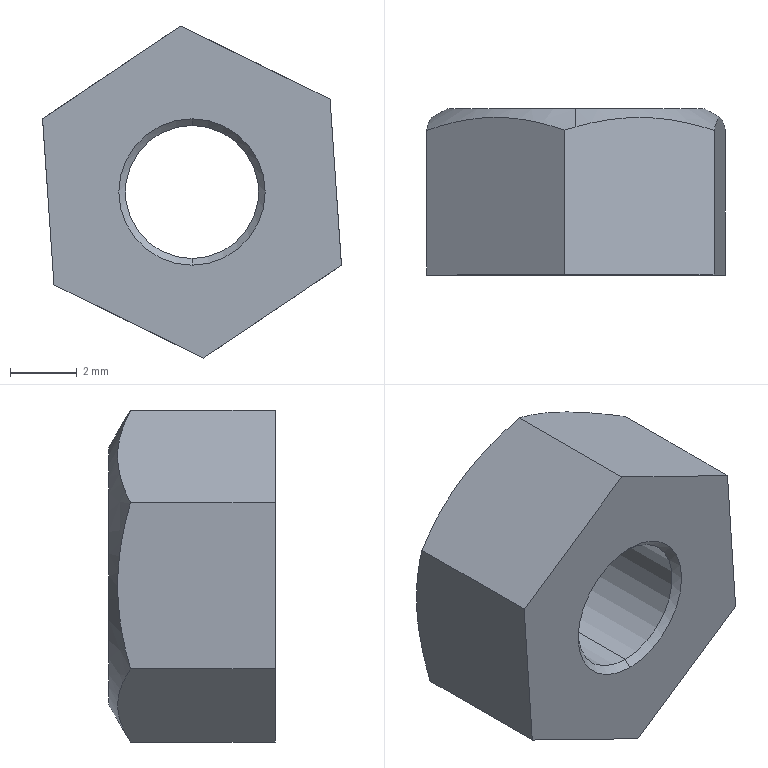Part | SolidWorks | features Chamfer 2, Extrusion 1, ICE 1 | 1 solid | 16 faces | box 8.983 x 5 x 9.976 mm | volume 257.478 mm3 | plane 8 | cone 6 | cylinder 2 | commonest cylinder face diameters 4 x2
STEP:
#1=CARTESIAN_POINT('',(0.,0.007874,0.07874));
#2=VERTEX_POINT('',#1);
#3=CARTESIAN_POINT('',(0.,0.007874,-0.07874));
#4=VERTEX_POINT('',#3);
#5=CARTESIAN_POINT('',(0.,0.007874,0.));
#6=DIRECTION('',(0.,-1.,0.));
#7=DIRECTION('',(0.,0.,1.));
#8=AXIS2_PLACEMENT_3D('',#5,#6,#7);
#9=CIRCLE('',#8,0.07874);
#10=EDGE_CURVE('',#2,#4,#9,.T.);
#11=ORIENTED_EDGE('',*,*,#10,.F.);
#12=CARTESIAN_POINT('',(0.,0.,0.08661));
#13=VERTEX_POINT('',#12);
#14=CARTESIAN_POINT('',(0.,0.,0.08661));
#15=DIRECTION('',(0.,-0.7071,0.7071));
#16=VECTOR('',#15,39.37);
#17=LINE('',#14,#16);
#18=EDGE_CURVE('',#2,#13,#17,.T.);
#19=ORIENTED_EDGE('',*,*,#18,.T.);
#20=CARTESIAN_POINT('',(0.,0.,-0.08661));
#21=VERTEX_POINT('',#20);
#22=CARTESIAN_POINT('',(0.,0.,0.));
#23=DIRECTION('',(0.,1.,0.));
#24=DIRECTION('',(0.,0.,1.));
#25=AXIS2_PLACEMENT_3D('',#22,#23,#24);
#26=CIRCLE('',#25,0.08661);
#27=EDGE_CURVE('',#21,#13,#26,.T.);
#28=ORIENTED_EDGE('',*,*,#27,.F.);
#29=CARTESIAN_POINT('',(0.,0.,-0.08661));
#30=DIRECTION('',(0.,-0.7071,-0.7071));
#31=VECTOR('',#30,39.37);
#32=LINE('',#29,#31);
#33=EDGE_CURVE('',#4,#21,#32,.T.);
#34=ORIENTED_EDGE('',*,*,#33,.F.);
#35=EDGE_LOOP('',(#11,#19,#28,#34));
#36=FACE_OUTER_BOUND('',#35,.T.);
#37=CARTESIAN_POINT('',(0.,0.,0.));
#38=DIRECTION('',(0.,-1.,0.));
#39=DIRECTION('',(0.,0.,-1.));
#40=AXIS2_PLACEMENT_3D('',#37,#38,#39);
#41=CONICAL_SURFACE('',#40,0.08661,0.7854);
#42=ADVANCED_FACE('',(#36),#41,.F.);
#43=CARTESIAN_POINT('',(0.,0.189,-0.07874));
#44=VERTEX_POINT('',#43);
#45=CARTESIAN_POINT('',(0.,0.189,0.07874));
#46=VERTEX_POINT('',#45);
#47=CARTESIAN_POINT('',(0.,0.189,0.));
#48=DIRECTION('',(0.,1.,0.));
#49=DIRECTION('',(0.,0.,1.));
#50=AXIS2_PLACEMENT_3D('',#47,#48,#49);
#51=CIRCLE('',#50,0.07874);
#52=EDGE_CURVE('',#44,#46,#51,.T.);
#53=ORIENTED_EDGE('',*,*,#52,.F.);
#54=CARTESIAN_POINT('',(0.,0.1969,-0.08661));
#55=VERTEX_POINT('',#54);
#56=CARTESIAN_POINT('',(0.,0.189,-0.07874));
#57=DIRECTION('',(0.,0.7071,-0.7071));
#58=VECTOR('',#57,39.37);
#59=LINE('',#56,#58);
#60=EDGE_CURVE('',#44,#55,#59,.T.);
#61=ORIENTED_EDGE('',*,*,#60,.T.);
#62=CARTESIAN_POINT('',(0.,0.1969,0.08661));
#63=VERTEX_POINT('',#62);
#64=CARTESIAN_POINT('',(0.,0.1969,0.));
#65=DIRECTION('',(0.,-1.,0.));
#66=DIRECTION('',(0.,0.,1.));
#67=AXIS2_PLACEMENT_3D('',#64,#65,#66);
#68=CIRCLE('',#67,0.08661);
#69=EDGE_CURVE('',#63,#55,#68,.T.);
#70=ORIENTED_EDGE('',*,*,#69,.F.);
#71=CARTESIAN_POINT('',(0.,0.189,0.07874));
#72=DIRECTION('',(0.,0.7071,0.7071));
#73=VECTOR('',#72,39.37);
#74=LINE('',#71,#73);
#75=EDGE_CURVE('',#46,#63,#74,.T.);
#76=ORIENTED_EDGE('',*,*,#75,.F.);
#77=EDGE_LOOP('',(#53,#61,#70,#76));
#78=FACE_OUTER_BOUND('',#77,.T.);
#79=CARTESIAN_POINT('',(0.,0.189,0.));
#80=DIRECTION('',(0.,1.,0.));
#81=DIRECTION('',(0.,0.,1.));
#82=AXIS2_PLACEMENT_3D('',#79,#80,#81);
#83=CONICAL_SURFACE('',#82,0.07874,0.7854);
#84=ADVANCED_FACE('',(#78),#83,.F.);
#85=CARTESIAN_POINT('',(0.,0.1969,-0.1523));
#86=VERTEX_POINT('',#85);
#87=CARTESIAN_POINT('',(0.,0.1969,0.1523));
#88=VERTEX_POINT('',#87);
#89=CARTESIAN_POINT('',(0.,0.1969,0.));
#90=DIRECTION('',(0.,1.,0.));
#91=DIRECTION('',(0.,0.,1.));
#92=AXIS2_PLACEMENT_3D('',#89,#90,#91);
#93=CIRCLE('',#92,0.1523);
#94=EDGE_CURVE('',#86,#88,#93,.T.);
#95=ORIENTED_EDGE('',*,*,#94,.F.);
#96=CARTESIAN_POINT('',(0.,0.1752,-0.1898));
#97=VERTEX_POINT('',#96);
#98=CARTESIAN_POINT('',(0.,0.1969,-0.1523));
#99=DIRECTION('',(0.,-0.5,-0.866));
#100=VECTOR('',#99,39.37);
#101=LINE('',#98,#100);
#102=EDGE_CURVE('',#86,#97,#101,.T.);
#103=ORIENTED_EDGE('',*,*,#102,.T.);
#104=CARTESIAN_POINT('',(-0.1633,0.1711,-0.1099));
#105=VERTEX_POINT('',#104);
#106=CARTESIAN_POINT('',(0.,0.1752,-0.1898));
#107=CARTESIAN_POINT('',(-0.02676,0.1828,-0.1767));
#108=CARTESIAN_POINT('',(-0.05395,0.1871,-0.1634));
#109=CARTESIAN_POINT('',(-0.1096,0.1855,-0.1362));
#110=CARTESIAN_POINT('',(-0.1367,0.1797,-0.1229));
#111=CARTESIAN_POINT('',(-0.1633,0.1711,-0.1099));
#112=B_SPLINE_CURVE_WITH_KNOTS('',3,(#106,#107,#108,#109,#110,#111),.UNSPECIFIED.,.F.,.F.,(4,2,4),(0.0003933,0.002722,0.00505),.UNSPECIFIED.);
#113=EDGE_CURVE('',#97,#105,#112,.T.);
#114=ORIENTED_EDGE('',*,*,#113,.T.);
#115=CARTESIAN_POINT('',(-0.1768,0.1711,0.08649));
#116=VERTEX_POINT('',#115);
#117=CARTESIAN_POINT('',(-0.1633,0.1711,-0.1099));
#118=CARTESIAN_POINT('',(-0.1655,0.1804,-0.07783));
#119=CARTESIAN_POINT('',(-0.1678,0.1863,-0.04529));
#120=CARTESIAN_POINT('',(-0.1712,0.1864,0.004801));
#121=CARTESIAN_POINT('',(-0.1724,0.1849,0.02148));
#122=CARTESIAN_POINT('',(-0.1746,0.1796,0.05425));
#123=CARTESIAN_POINT('',(-0.1757,0.1758,0.07043));
#124=CARTESIAN_POINT('',(-0.1768,0.1711,0.08649));
#125=B_SPLINE_CURVE_WITH_KNOTS('',3,(#117,#118,#119,#120,#121,#122,#123,#124),.UNSPECIFIED.,.F.,.F.,(4,2,2,4),(0.000000207,0.002525,0.003788,0.00505),.UNSPECIFIED.);
#126=EDGE_CURVE('',#105,#116,#125,.T.);
#127=ORIENTED_EDGE('',*,*,#126,.T.);
#128=CARTESIAN_POINT('',(-0.01352,0.1711,0.1964));
#129=VERTEX_POINT('',#128);
#130=CARTESIAN_POINT('',(-0.1768,0.1711,0.08649));
#131=CARTESIAN_POINT('',(-0.1502,0.1804,0.1044));
#132=CARTESIAN_POINT('',(-0.1231,0.1863,0.1226));
#133=CARTESIAN_POINT('',(-0.08145,0.1864,0.1507));
#134=CARTESIAN_POINT('',(-0.06758,0.1849,0.16));
#135=CARTESIAN_POINT('',(-0.04033,0.1796,0.1783));
#136=CARTESIAN_POINT('',(-0.02687,0.1758,0.1874));
#137=CARTESIAN_POINT('',(-0.01352,0.1711,0.1964));
#138=B_SPLINE_CURVE_WITH_KNOTS('',3,(#130,#131,#132,#133,#134,#135,#136,#137),.UNSPECIFIED.,.F.,.F.,(4,2,2,4),(0.000000248,0.002525,0.003788,0.00505),.UNSPECIFIED.);
#139=EDGE_CURVE('',#116,#129,#138,.T.);
#140=ORIENTED_EDGE('',*,*,#139,.T.);
#141=CARTESIAN_POINT('',(0.,0.1752,0.1898));
#142=VERTEX_POINT('',#141);
#143=CARTESIAN_POINT('',(-0.01352,0.1711,0.1964));
#144=CARTESIAN_POINT('',(-0.009023,0.1726,0.1942));
#145=CARTESIAN_POINT('',(-0.004517,0.174,0.192));
#146=CARTESIAN_POINT('',(0.,0.1752,0.1898));
#147=B_SPLINE_CURVE_WITH_KNOTS('',3,(#143,#144,#145,#146),.UNSPECIFIED.,.F.,.F.,(4,4),(0.00000023,0.0003933),.UNSPECIFIED.);
#148=EDGE_CURVE('',#129,#142,#147,.T.);
#149=ORIENTED_EDGE('',*,*,#148,.T.);
#150=CARTESIAN_POINT('',(0.,0.1969,0.1523));
#151=DIRECTION('',(0.,-0.5,0.866));
#152=VECTOR('',#151,39.37);
#153=LINE('',#150,#152);
#154=EDGE_CURVE('',#88,#142,#153,.T.);
#155=ORIENTED_EDGE('',*,*,#154,.F.);
#156=EDGE_LOOP('',(#95,#103,#114,#127,#140,#149,#155));
#157=FACE_OUTER_BOUND('',#156,.T.);
#158=CARTESIAN_POINT('',(0.,0.1969,0.));
#159=DIRECTION('',(0.,-1.,0.));
#160=DIRECTION('',(0.,0.,1.));
#161=AXIS2_PLACEMENT_3D('',#158,#159,#160);
#162=CONICAL_SURFACE('',#161,0.1523,1.047);
#163=ADVANCED_FACE('',(#157),#162,.T.);
#164=ORIENTED_EDGE('',*,*,#52,.T.);
#165=CARTESIAN_POINT('',(0.,0.1969,0.07874));
#166=DIRECTION('',(0.,-1.,0.));
#167=VECTOR('',#166,39.37);
#168=LINE('',#165,#167);
#169=EDGE_CURVE('',#46,#2,#168,.T.);
#170=ORIENTED_EDGE('',*,*,#169,.T.);
#171=ORIENTED_EDGE('',*,*,#10,.T.);
#172=CARTESIAN_POINT('',(0.,0.1969,-0.07874));
#173=DIRECTION('',(0.,-1.,0.));
#174=VECTOR('',#173,39.37);
#175=LINE('',#172,#174);
#176=EDGE_CURVE('',#44,#4,#175,.T.);
#177=ORIENTED_EDGE('',*,*,#176,.F.);
#178=EDGE_LOOP('',(#164,#170,#171,#177));
#179=FACE_OUTER_BOUND('',#178,.T.);
#180=CARTESIAN_POINT('',(0.,0.1969,0.));
#181=DIRECTION('',(0.,-1.,0.));
#182=DIRECTION('',(0.,0.,-1.));
#183=AXIS2_PLACEMENT_3D('',#180,#181,#182);
#184=CYLINDRICAL_SURFACE('',#183,0.07874);
#185=ADVANCED_FACE('',(#179),#184,.F.);
#186=ORIENTED_EDGE('',*,*,#69,.T.);
#187=CARTESIAN_POINT('',(0.,0.1969,0.));
#188=DIRECTION('',(0.,-1.,0.));
#189=DIRECTION('',(0.,0.,1.));
#190=AXIS2_PLACEMENT_3D('',#187,#188,#189);
#191=CIRCLE('',#190,0.08661);
#192=EDGE_CURVE('',#55,#63,#191,.T.);
#193=ORIENTED_EDGE('',*,*,#192,.T.);
#194=EDGE_LOOP('',(#186,#193));
#195=FACE_BOUND('',#194,.T.);
#196=CARTESIAN_POINT('',(0.,0.1969,0.));
#197=DIRECTION('',(0.,1.,0.));
#198=DIRECTION('',(0.,0.,1.));
#199=AXIS2_PLACEMENT_3D('',#196,#197,#198);
#200=CIRCLE('',#199,0.1523);
#201=EDGE_CURVE('',#88,#86,#200,.T.);
#202=ORIENTED_EDGE('',*,*,#201,.T.);
#203=ORIENTED_EDGE('',*,*,#94,.T.);
#204=EDGE_LOOP('',(#202,#203));
#205=FACE_OUTER_BOUND('',#204,.T.);
#206=CARTESIAN_POINT('',(0.,0.1969,0.));
#207=DIRECTION('',(0.,1.,0.));
#208=DIRECTION('',(0.,0.,1.));
#209=AXIS2_PLACEMENT_3D('',#206,#207,#208);
#210=PLANE('',#209);
#211=ADVANCED_FACE('',(#195,#205),#210,.T.);
#212=ORIENTED_EDGE('',*,*,#148,.F.);
#213=CARTESIAN_POINT('',(-0.01352,0.,0.1964));
#214=VERTEX_POINT('',#213);
#215=CARTESIAN_POINT('',(-0.01352,0.1969,0.1964));
#216=DIRECTION('',(0.,-1.,0.));
#217=VECTOR('',#216,39.37);
#218=LINE('',#215,#217);
#219=EDGE_CURVE('',#129,#214,#218,.T.);
#220=ORIENTED_EDGE('',*,*,#219,.T.);
#221=CARTESIAN_POINT('',(0.1633,0.,0.1099));
#222=VERTEX_POINT('',#221);
#223=CARTESIAN_POINT('',(-0.01352,0.,0.1964));
#224=DIRECTION('',(0.8983,0.,-0.4393));
#225=VECTOR('',#224,39.37);
#226=LINE('',#223,#225);
#227=EDGE_CURVE('',#214,#222,#226,.T.);
#228=ORIENTED_EDGE('',*,*,#227,.T.);
#229=CARTESIAN_POINT('',(0.1633,0.1711,0.1099));
#230=VERTEX_POINT('',#229);
#231=CARTESIAN_POINT('',(0.1633,0.1969,0.1099));
#232=DIRECTION('',(0.,-1.,0.));
#233=VECTOR('',#232,39.37);
#234=LINE('',#231,#233);
#235=EDGE_CURVE('',#230,#222,#234,.T.);
#236=ORIENTED_EDGE('',*,*,#235,.F.);
#237=CARTESIAN_POINT('',(0.,0.1752,0.1898));
#238=CARTESIAN_POINT('',(0.02676,0.1828,0.1767));
#239=CARTESIAN_POINT('',(0.05395,0.1871,0.1634));
#240=CARTESIAN_POINT('',(0.1096,0.1855,0.1362));
#241=CARTESIAN_POINT('',(0.1367,0.1797,0.1229));
#242=CARTESIAN_POINT('',(0.1633,0.1711,0.1099));
#243=B_SPLINE_CURVE_WITH_KNOTS('',3,(#237,#238,#239,#240,#241,#242),.UNSPECIFIED.,.F.,.F.,(4,2,4),(0.0003933,0.002722,0.00505),.UNSPECIFIED.);
#244=EDGE_CURVE('',#142,#230,#243,.T.);
#245=ORIENTED_EDGE('',*,*,#244,.F.);
#246=EDGE_LOOP('',(#212,#220,#228,#236,#245));
#247=FACE_OUTER_BOUND('',#246,.T.);
#248=CARTESIAN_POINT('',(-0.01352,0.1969,0.1964));
#249=DIRECTION('',(-0.4393,0.,-0.8983));
#250=DIRECTION('',(-0.8983,0.,0.4393));
#251=AXIS2_PLACEMENT_3D('',#248,#249,#250);
#252=PLANE('',#251);
#253=ADVANCED_FACE('',(#247),#252,.F.);
#254=CARTESIAN_POINT('',(0.1768,0.1711,-0.08649));
#255=VERTEX_POINT('',#254);
#256=CARTESIAN_POINT('',(0.1633,0.1711,0.1099));
#257=CARTESIAN_POINT('',(0.1655,0.1804,0.07783));
#258=CARTESIAN_POINT('',(0.1678,0.1863,0.04529));
#259=CARTESIAN_POINT('',(0.1712,0.1864,-0.004801));
#260=CARTESIAN_POINT('',(0.1724,0.1849,-0.02148));
#261=CARTESIAN_POINT('',(0.1746,0.1796,-0.05425));
#262=CARTESIAN_POINT('',(0.1757,0.1758,-0.07043));
#263=CARTESIAN_POINT('',(0.1768,0.1711,-0.08649));
#264=B_SPLINE_CURVE_WITH_KNOTS('',3,(#256,#257,#258,#259,#260,#261,#262,#263),.UNSPECIFIED.,.F.,.F.,(4,2,2,4),(0.000000207,0.002525,0.003788,0.00505),.UNSPECIFIED.);
#265=EDGE_CURVE('',#230,#255,#264,.T.);
#266=ORIENTED_EDGE('',*,*,#265,.F.);
#267=ORIENTED_EDGE('',*,*,#235,.T.);
#268=CARTESIAN_POINT('',(0.1768,0.,-0.08649));
#269=VERTEX_POINT('',#268);
#270=CARTESIAN_POINT('',(0.1633,0.,0.1099));
#271=DIRECTION('',(0.06867,0.,-0.9976));
#272=VECTOR('',#271,39.37);
#273=LINE('',#270,#272);
#274=EDGE_CURVE('',#222,#269,#273,.T.);
#275=ORIENTED_EDGE('',*,*,#274,.T.);
#276=CARTESIAN_POINT('',(0.1768,0.1969,-0.08649));
#277=DIRECTION('',(0.,-1.,0.));
#278=VECTOR('',#277,39.37);
#279=LINE('',#276,#278);
#280=EDGE_CURVE('',#255,#269,#279,.T.);
#281=ORIENTED_EDGE('',*,*,#280,.F.);
#282=EDGE_LOOP('',(#266,#267,#275,#281));
#283=FACE_OUTER_BOUND('',#282,.T.);
#284=CARTESIAN_POINT('',(0.1633,0.1969,0.1099));
#285=DIRECTION('',(-0.9976,0.,-0.06867));
#286=DIRECTION('',(-0.06867,0.,0.9976));
#287=AXIS2_PLACEMENT_3D('',#284,#285,#286);
#288=PLANE('',#287);
#289=ADVANCED_FACE('',(#283),#288,.F.);
#290=CARTESIAN_POINT('',(0.01352,0.1711,-0.1964));
#291=VERTEX_POINT('',#290);
#292=CARTESIAN_POINT('',(0.1768,0.1711,-0.08649));
#293=CARTESIAN_POINT('',(0.1502,0.1804,-0.1044));
#294=CARTESIAN_POINT('',(0.1231,0.1863,-0.1226));
#295=CARTESIAN_POINT('',(0.08145,0.1864,-0.1507));
#296=CARTESIAN_POINT('',(0.06758,0.1849,-0.16));
#297=CARTESIAN_POINT('',(0.04033,0.1796,-0.1783));
#298=CARTESIAN_POINT('',(0.02687,0.1758,-0.1874));
#299=CARTESIAN_POINT('',(0.01352,0.1711,-0.1964));
#300=B_SPLINE_CURVE_WITH_KNOTS('',3,(#292,#293,#294,#295,#296,#297,#298,#299),.UNSPECIFIED.,.F.,.F.,(4,2,2,4),(0.000000248,0.002525,0.003788,0.00505),.UNSPECIFIED.);
#301=EDGE_CURVE('',#255,#291,#300,.T.);
#302=ORIENTED_EDGE('',*,*,#301,.F.);
#303=ORIENTED_EDGE('',*,*,#280,.T.);
#304=CARTESIAN_POINT('',(0.01352,0.,-0.1964));
#305=VERTEX_POINT('',#304);
#306=CARTESIAN_POINT('',(0.1768,0.,-0.08649));
#307=DIRECTION('',(-0.8296,0.,-0.5583));
#308=VECTOR('',#307,39.37);
#309=LINE('',#306,#308);
#310=EDGE_CURVE('',#269,#305,#309,.T.);
#311=ORIENTED_EDGE('',*,*,#310,.T.);
#312=CARTESIAN_POINT('',(0.01352,0.1969,-0.1964));
#313=DIRECTION('',(0.,-1.,0.));
#314=VECTOR('',#313,39.37);
#315=LINE('',#312,#314);
#316=EDGE_CURVE('',#291,#305,#315,.T.);
#317=ORIENTED_EDGE('',*,*,#316,.F.);
#318=EDGE_LOOP('',(#302,#303,#311,#317));
#319=FACE_OUTER_BOUND('',#318,.T.);
#320=CARTESIAN_POINT('',(0.1768,0.1969,-0.08649));
#321=DIRECTION('',(-0.5583,0.,0.8296));
#322=DIRECTION('',(0.8296,0.,0.5583));
#323=AXIS2_PLACEMENT_3D('',#320,#321,#322);
#324=PLANE('',#323);
#325=ADVANCED_FACE('',(#319),#324,.F.);
#326=CARTESIAN_POINT('',(0.01352,0.1711,-0.1964));
#327=CARTESIAN_POINT('',(0.009023,0.1726,-0.1942));
#328=CARTESIAN_POINT('',(0.004517,0.174,-0.192));
#329=CARTESIAN_POINT('',(0.,0.1752,-0.1898));
#330=B_SPLINE_CURVE_WITH_KNOTS('',3,(#326,#327,#328,#329),.UNSPECIFIED.,.F.,.F.,(4,4),(0.00000023,0.0003933),.UNSPECIFIED.);
#331=EDGE_CURVE('',#291,#97,#330,.T.);
#332=ORIENTED_EDGE('',*,*,#331,.F.);
#333=ORIENTED_EDGE('',*,*,#316,.T.);
#334=CARTESIAN_POINT('',(-0.1633,0.,-0.1099));
#335=VERTEX_POINT('',#334);
#336=CARTESIAN_POINT('',(0.01352,0.,-0.1964));
#337=DIRECTION('',(-0.8983,0.,0.4393));
#338=VECTOR('',#337,39.37);
#339=LINE('',#336,#338);
#340=EDGE_CURVE('',#305,#335,#339,.T.);
#341=ORIENTED_EDGE('',*,*,#340,.T.);
#342=CARTESIAN_POINT('',(-0.1633,0.1969,-0.1099));
#343=DIRECTION('',(0.,-1.,0.));
#344=VECTOR('',#343,39.37);
#345=LINE('',#342,#344);
#346=EDGE_CURVE('',#105,#335,#345,.T.);
#347=ORIENTED_EDGE('',*,*,#346,.F.);
#348=ORIENTED_EDGE('',*,*,#113,.F.);
#349=EDGE_LOOP('',(#332,#333,#341,#347,#348));
#350=FACE_OUTER_BOUND('',#349,.T.);
#351=CARTESIAN_POINT('',(0.01352,0.1969,-0.1964));
#352=DIRECTION('',(0.4393,0.,0.8983));
#353=DIRECTION('',(0.8983,0.,-0.4393));
#354=AXIS2_PLACEMENT_3D('',#351,#352,#353);
#355=PLANE('',#354);
#356=ADVANCED_FACE('',(#350),#355,.F.);
#357=ORIENTED_EDGE('',*,*,#126,.F.);
#358=ORIENTED_EDGE('',*,*,#346,.T.);
#359=CARTESIAN_POINT('',(-0.1768,0.,0.08649));
#360=VERTEX_POINT('',#359);
#361=CARTESIAN_POINT('',(-0.1633,0.,-0.1099));
#362=DIRECTION('',(-0.06867,0.,0.9976));
#363=VECTOR('',#362,39.37);
#364=LINE('',#361,#363);
#365=EDGE_CURVE('',#335,#360,#364,.T.);
#366=ORIENTED_EDGE('',*,*,#365,.T.);
#367=CARTESIAN_POINT('',(-0.1768,0.1969,0.08649));
#368=DIRECTION('',(0.,-1.,0.));
#369=VECTOR('',#368,39.37);
#370=LINE('',#367,#369);
#371=EDGE_CURVE('',#116,#360,#370,.T.);
#372=ORIENTED_EDGE('',*,*,#371,.F.);
#373=EDGE_LOOP('',(#357,#358,#366,#372));
#374=FACE_OUTER_BOUND('',#373,.T.);
#375=CARTESIAN_POINT('',(-0.1633,0.1969,-0.1099));
#376=DIRECTION('',(0.9976,0.,0.06867));
#377=DIRECTION('',(0.06867,0.,-0.9976));
#378=AXIS2_PLACEMENT_3D('',#375,#376,#377);
#379=PLANE('',#378);
#380=ADVANCED_FACE('',(#374),#379,.F.);
#381=ORIENTED_EDGE('',*,*,#139,.F.);
#382=ORIENTED_EDGE('',*,*,#371,.T.);
#383=CARTESIAN_POINT('',(-0.1768,0.,0.08649));
#384=DIRECTION('',(0.8296,0.,0.5583));
#385=VECTOR('',#384,39.37);
#386=LINE('',#383,#385);
#387=EDGE_CURVE('',#360,#214,#386,.T.);
#388=ORIENTED_EDGE('',*,*,#387,.T.);
#389=ORIENTED_EDGE('',*,*,#219,.F.);
#390=EDGE_LOOP('',(#381,#382,#388,#389));
#391=FACE_OUTER_BOUND('',#390,.T.);
#392=CARTESIAN_POINT('',(-0.1768,0.1969,0.08649));
#393=DIRECTION('',(0.5583,0.,-0.8296));
#394=DIRECTION('',(-0.8296,0.,-0.5583));
#395=AXIS2_PLACEMENT_3D('',#392,#393,#394);
#396=PLANE('',#395);
#397=ADVANCED_FACE('',(#391),#396,.F.);
#398=ORIENTED_EDGE('',*,*,#27,.T.);
#399=CARTESIAN_POINT('',(0.,0.,0.));
#400=DIRECTION('',(0.,1.,0.));
#401=DIRECTION('',(0.,0.,1.));
#402=AXIS2_PLACEMENT_3D('',#399,#400,#401);
#403=CIRCLE('',#402,0.08661);
#404=EDGE_CURVE('',#13,#21,#403,.T.);
#405=ORIENTED_EDGE('',*,*,#404,.T.);
#406=EDGE_LOOP('',(#398,#405));
#407=FACE_BOUND('',#406,.T.);
#408=ORIENTED_EDGE('',*,*,#227,.F.);
#409=ORIENTED_EDGE('',*,*,#387,.F.);
#410=ORIENTED_EDGE('',*,*,#365,.F.);
#411=ORIENTED_EDGE('',*,*,#340,.F.);
#412=ORIENTED_EDGE('',*,*,#310,.F.);
#413=ORIENTED_EDGE('',*,*,#274,.F.);
#414=EDGE_LOOP('',(#408,#409,#410,#411,#412,#413));
#415=FACE_OUTER_BOUND('',#414,.T.);
#416=CARTESIAN_POINT('',(0.,0.,0.));
#417=DIRECTION('',(0.,1.,0.));
#418=DIRECTION('',(0.,0.,1.));
#419=AXIS2_PLACEMENT_3D('',#416,#417,#418);
#420=PLANE('',#419);
#421=ADVANCED_FACE('',(#407,#415),#420,.F.);
#422=ORIENTED_EDGE('',*,*,#169,.F.);
#423=CARTESIAN_POINT('',(0.,0.189,0.));
#424=DIRECTION('',(0.,1.,0.));
#425=DIRECTION('',(0.,0.,1.));
#426=AXIS2_PLACEMENT_3D('',#423,#424,#425);
#427=CIRCLE('',#426,0.07874);
#428=EDGE_CURVE('',#46,#44,#427,.T.);
#429=ORIENTED_EDGE('',*,*,#428,.T.);
#430=ORIENTED_EDGE('',*,*,#176,.T.);
#431=CARTESIAN_POINT('',(0.,0.007874,0.));
#432=DIRECTION('',(0.,-1.,0.));
#433=DIRECTION('',(0.,0.,1.));
#434=AXIS2_PLACEMENT_3D('',#431,#432,#433);
#435=CIRCLE('',#434,0.07874);
#436=EDGE_CURVE('',#4,#2,#435,.T.);
#437=ORIENTED_EDGE('',*,*,#436,.T.);
#438=EDGE_LOOP('',(#422,#429,#430,#437));
#439=FACE_OUTER_BOUND('',#438,.T.);
#440=CARTESIAN_POINT('',(0.,0.1969,0.));
#441=DIRECTION('',(0.,-1.,0.));
#442=DIRECTION('',(0.,0.,-1.));
#443=AXIS2_PLACEMENT_3D('',#440,#441,#442);
#444=CYLINDRICAL_SURFACE('',#443,0.07874);
#445=ADVANCED_FACE('',(#439),#444,.F.);
#446=ORIENTED_EDGE('',*,*,#102,.F.);
#447=ORIENTED_EDGE('',*,*,#201,.F.);
#448=ORIENTED_EDGE('',*,*,#154,.T.);
#449=ORIENTED_EDGE('',*,*,#244,.T.);
#450=ORIENTED_EDGE('',*,*,#265,.T.);
#451=ORIENTED_EDGE('',*,*,#301,.T.);
#452=ORIENTED_EDGE('',*,*,#331,.T.);
#453=EDGE_LOOP('',(#446,#447,#448,#449,#450,#451,#452));
#454=FACE_OUTER_BOUND('',#453,.T.);
#455=CARTESIAN_POINT('',(0.,0.1969,0.));
#456=DIRECTION('',(0.,-1.,0.));
#457=DIRECTION('',(0.,0.,1.));
#458=AXIS2_PLACEMENT_3D('',#455,#456,#457);
#459=CONICAL_SURFACE('',#458,0.1523,1.047);
#460=ADVANCED_FACE('',(#454),#459,.T.);
#461=ORIENTED_EDGE('',*,*,#60,.F.);
#462=ORIENTED_EDGE('',*,*,#428,.F.);
#463=ORIENTED_EDGE('',*,*,#75,.T.);
#464=ORIENTED_EDGE('',*,*,#192,.F.);
#465=EDGE_LOOP('',(#461,#462,#463,#464));
#466=FACE_OUTER_BOUND('',#465,.T.);
#467=CARTESIAN_POINT('',(0.,0.189,0.));
#468=DIRECTION('',(0.,1.,0.));
#469=DIRECTION('',(0.,0.,1.));
#470=AXIS2_PLACEMENT_3D('',#467,#468,#469);
#471=CONICAL_SURFACE('',#470,0.07874,0.7854);
#472=ADVANCED_FACE('',(#466),#471,.F.);
#473=ORIENTED_EDGE('',*,*,#18,.F.);
#474=ORIENTED_EDGE('',*,*,#436,.F.);
#475=ORIENTED_EDGE('',*,*,#33,.T.);
#476=ORIENTED_EDGE('',*,*,#404,.F.);
#477=EDGE_LOOP('',(#473,#474,#475,#476));
#478=FACE_OUTER_BOUND('',#477,.T.);
#479=CARTESIAN_POINT('',(0.,0.,0.));
#480=DIRECTION('',(0.,-1.,0.));
#481=DIRECTION('',(0.,0.,-1.));
#482=AXIS2_PLACEMENT_3D('',#479,#480,#481);
#483=CONICAL_SURFACE('',#482,0.08661,0.7854);
#484=ADVANCED_FACE('',(#478),#483,.F.);
#485=CLOSED_SHELL('',(#42,#84,#163,#185,#211,#253,#289,#325,#356,#380,#397,#421,#445,#460,#472,#484));
#486=MANIFOLD_SOLID_BREP('',#485);
#487=CARTESIAN_POINT('',(0.,0.,0.));
#488=DIRECTION('',(0.,0.,1.));
#489=DIRECTION('',(1.,0.,0.));
#490=AXIS2_PLACEMENT_3D('',#487,#488,#489);
#491=(LENGTH_UNIT()NAMED_UNIT(*)SI_UNIT($,.METRE.));
#492=LENGTH_MEASURE_WITH_UNIT(LENGTH_MEASURE(0.0254),#491);
#493=DIMENSIONAL_EXPONENTS(1.,0.,0.,0.,0.,0.,0.);
#494=(CONVERSION_BASED_UNIT('INCH',#492)LENGTH_UNIT()NAMED_UNIT(#493));
#495=UNCERTAINTY_MEASURE_WITH_UNIT(LENGTH_MEASURE(0.00001),#494,'','');
#496=(NAMED_UNIT(*)PLANE_ANGLE_UNIT()SI_UNIT($,.RADIAN.));
#497=(NAMED_UNIT(*)SI_UNIT($,.STERADIAN.)SOLID_ANGLE_UNIT());
#498=(GEOMETRIC_REPRESENTATION_CONTEXT(3)GLOBAL_UNCERTAINTY_ASSIGNED_CONTEXT((#495))GLOBAL_UNIT_ASSIGNED_CONTEXT((#494,#496,#497))REPRESENTATION_CONTEXT('',''));
#499=ADVANCED_BREP_SHAPE_REPRESENTATION('',(#486,#490),#498);